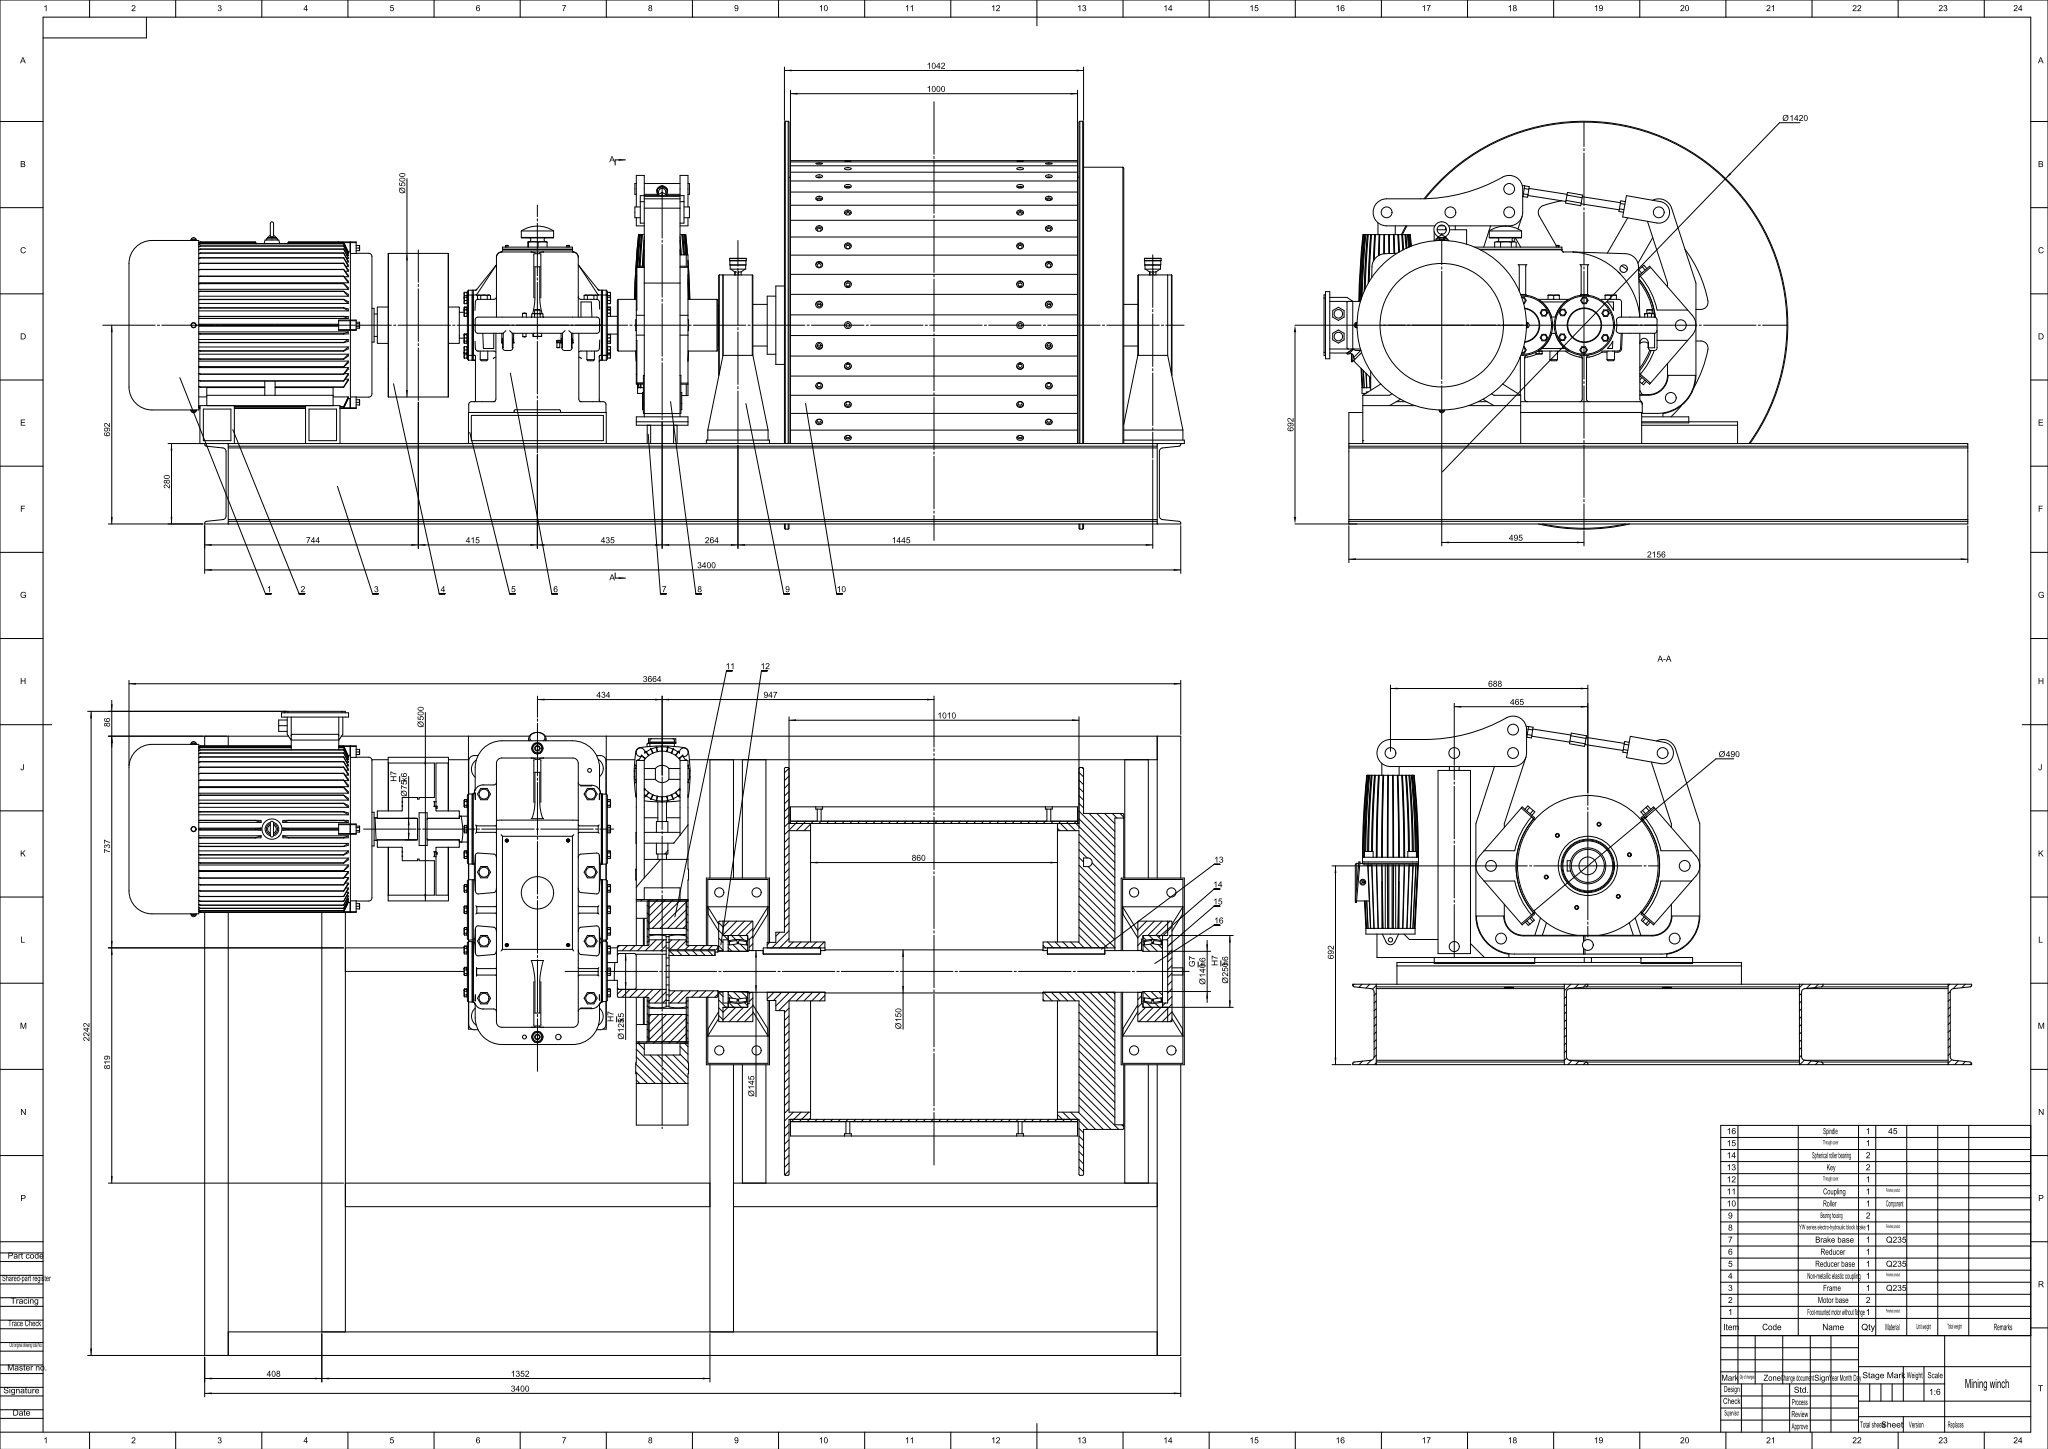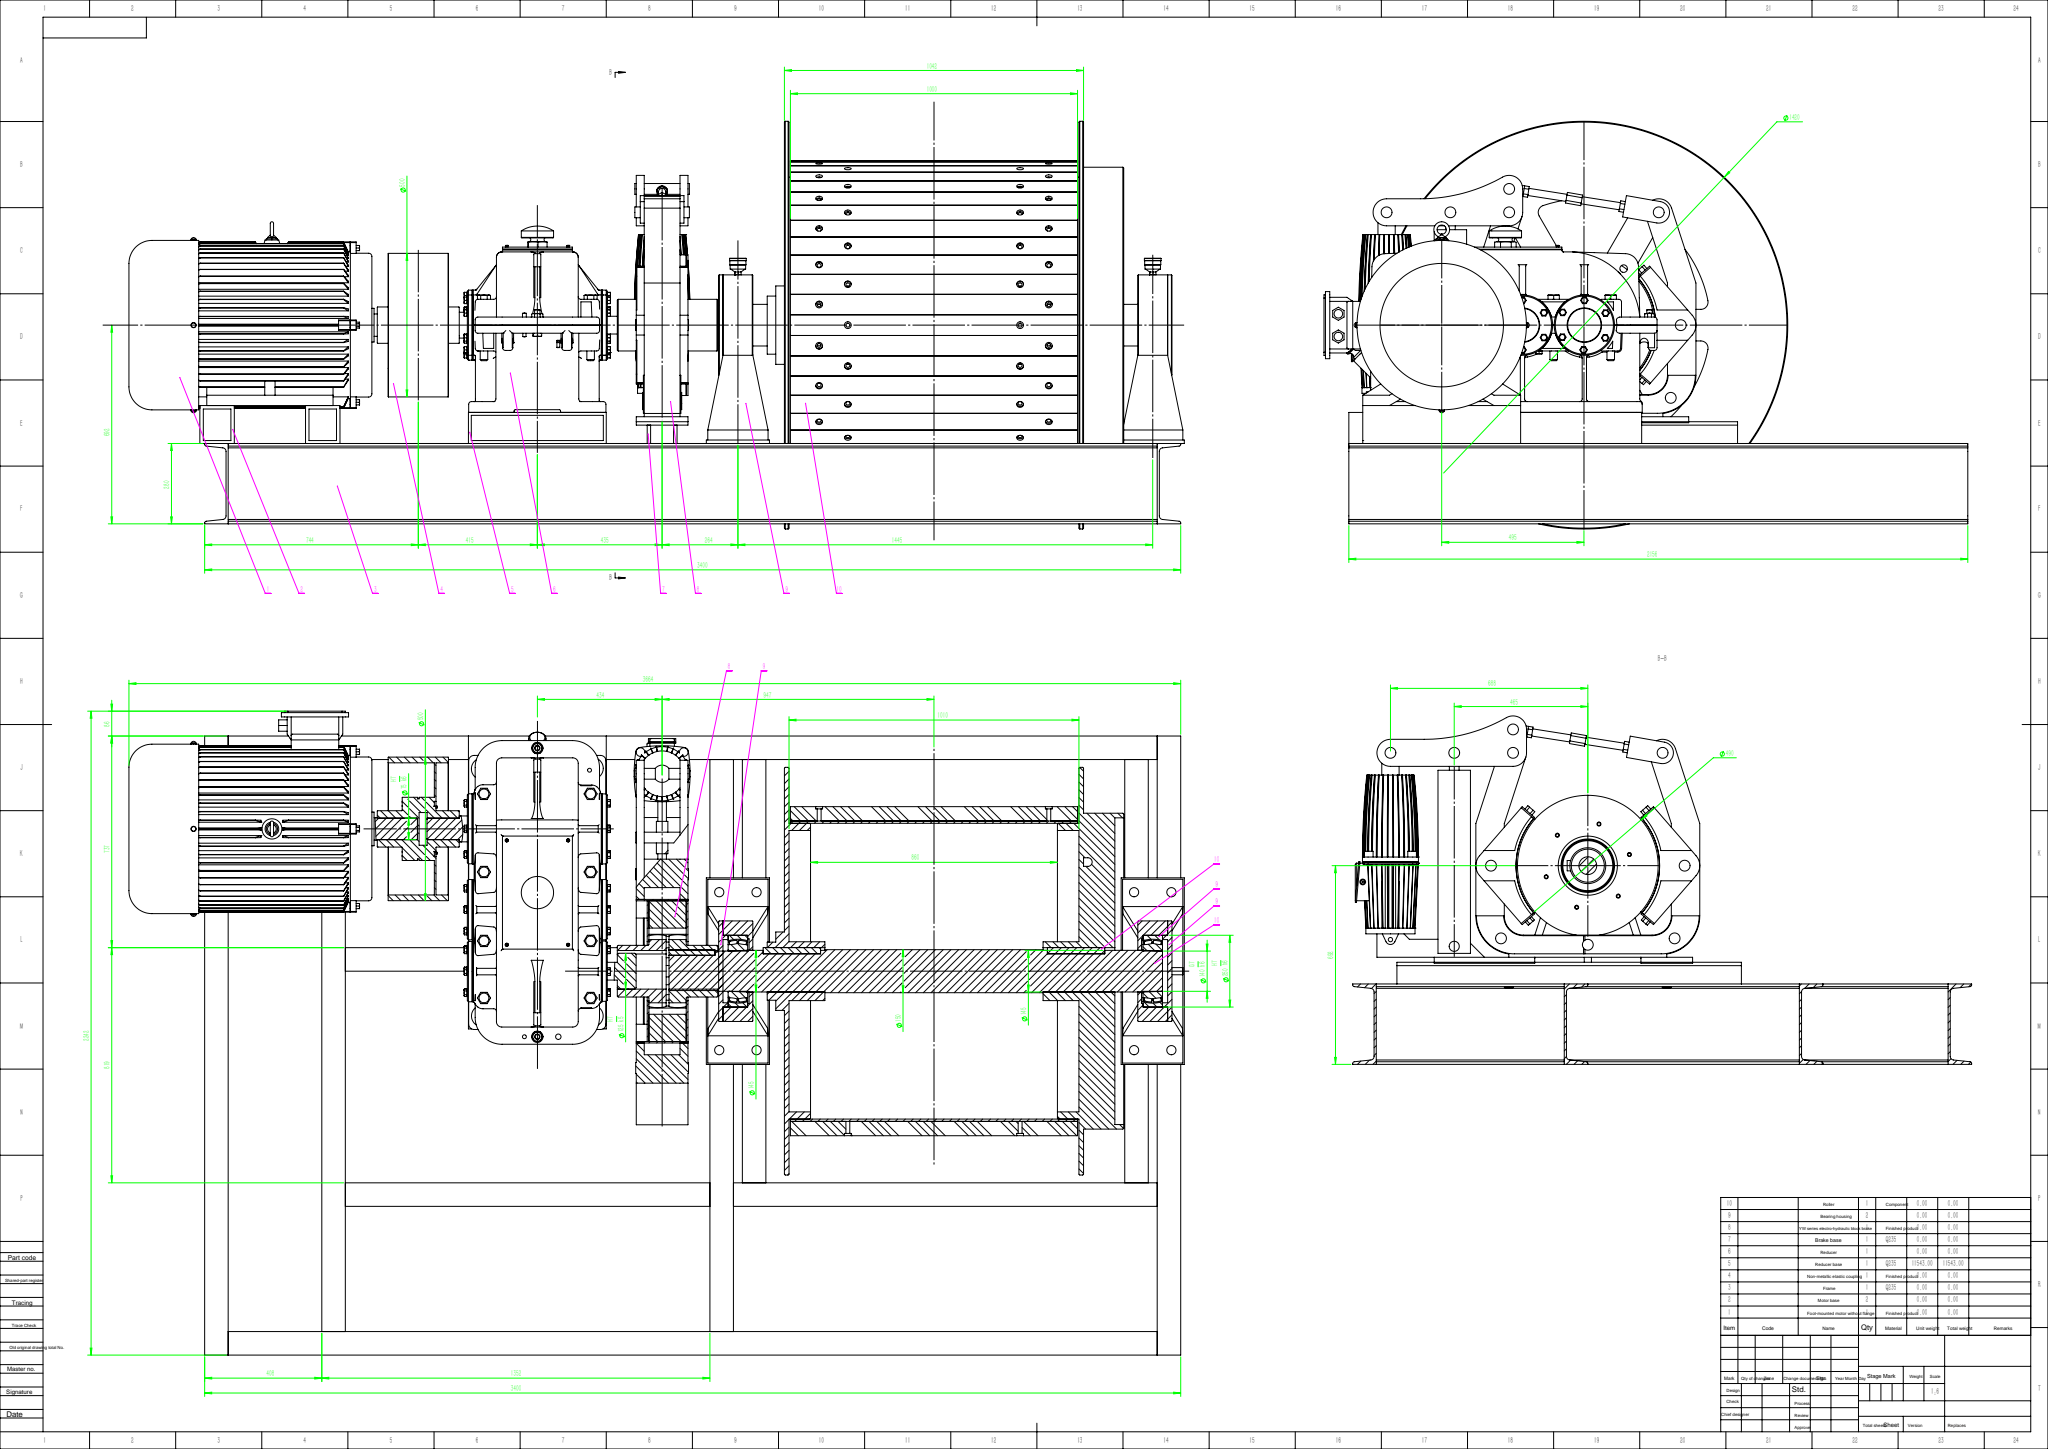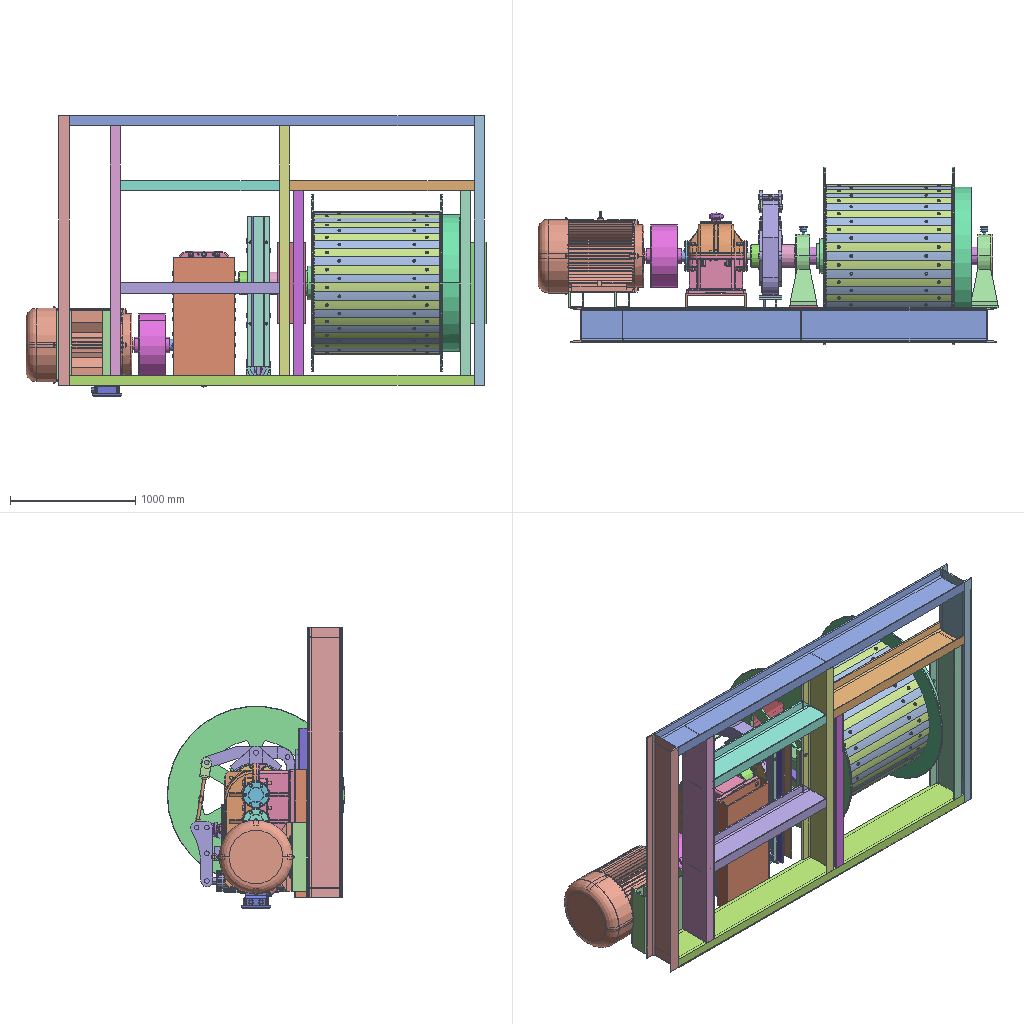Assembly | SolidWorks | 66 different items | 167 placed | box 3676 x 1420 x 2242 mm
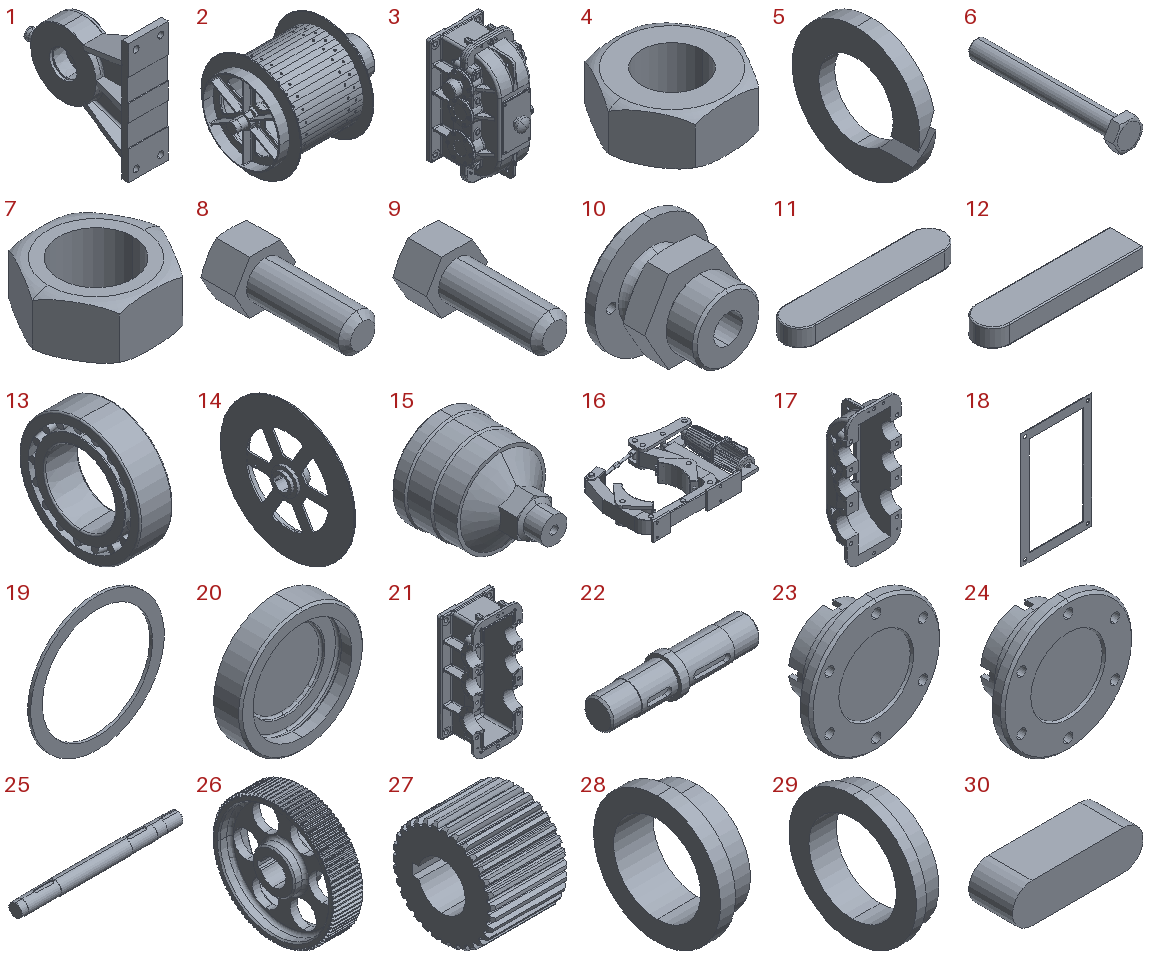Parts list (item | name | quantity | parent item | size | volume | features):
1 | (subassembly) | x2 | - | 210 x 633 x 640 mm | 18025314 mm3 | -
2 | (subassembly) | x1 | - | 1899 x 1420 x 1420 mm | 323309066 mm3 | features ReferencePattern 24, LocalCirPattern 1
3 | (subassembly) | x1 | - | - | 87002106 mm3 | features ReferencePattern 45, CompositeCurve 27, MirrorCompFeat 4, LocalCirPattern 3, AEMSimFeature 1
4 | - | x2 | in 3 | 38.971 x 33.75 x 15 mm | 10501 mm3 | features Extrusion 1, RevCut 1, Scale 1
5 | - | x8 | in 3 | 3 x 24 x 24 mm | 848.529 mm3 | features ICE 1, Revolution 1
6 | - | x8 | in 3 | 45.466 x 228.75 x 39.375 mm | 135169 mm3 | features Chamfer 1, Extrusion 1, ICE 1, RevCut 1, Scale 1
7 | - | x8 | in 3 | 24.249 x 21 x 10 mm | 2242 mm3 | features Extrusion 1, ICE 1, RevCut 1
8 | - | x2 | in 3 | 10 x 22 x 8.66 mm | 745.342 mm3 | features ICE 2, BlendCut 1, Chamfer 1, RevCut 1, Revolution 1
9 | - | x2 | in 3 | 10 x 22 x 8.66 mm | 755.833 mm3 | features ICE 2, Revolution 2, BlendCut 1, Chamfer 1, Fillet 1, RevCut 1
10 | - | x1 | in 3 | 90 x 69.375 x 90 mm | 178103 mm3 | features Chamfer 2, ICE 2, RevCut 1, Revolution 1, Scale 1
11 | - | x2 | in 2 | 200 x 40 x 22 mm | 168172 mm3 | features Extrusion 1, Fillet 1
12 | - | x1 | in 2 | 160 x 36 x 20 mm | 112209 mm3 | features Extrusion 1, Fillet 1
13 | - | x2 | in 1 | 68 x 250 x 250 mm | 1755852 mm3 | features Revolution 3, CirPattern 1, Fillet 1, MirrorPattern 1
14 | - | x1 | in 2 | 201 x 1420 x 1420 mm | 29509148 mm3 | features ICE 5, CirPattern 2, Chamfer 1, Fillet 1, RevCut 1, Revolution 1
15 | - | x2 | in 1 | 58 x 70 x 58 mm | 93422 mm3 | features Boss 1, Revolution 1
16 | - | x1 | - | 1200 x 861.523 x 195 mm | 52258785 mm3 | features Boss 43, Fillet 5, MirrorPattern 5, Cut 4, CombineBodies 3, CirPattern 2, Revolution 2, Extrusion 1, MirrorSolid 1
17 | - | x1 | in 3 | 446.25 x 262.5 x 1058 mm | 19685797 mm3 | features Fillet 30, ICE 30, MirrorPattern 4, RevCut 3, Revolution 3, Sculpt 2, Extrusion 1, Scale 1
18 | - | x1 | in 3 | 241.875 x 1.875 x 393.75 mm | 60360 mm3 | features Extrusion 1, Scale 1
19 | - | x1 | in 3 | 46 x 1 x 46 mm | 527.788 mm3 | features Revolution 1
20 | - | x1 | in 3 | 112.5 x 41.25 x 112.5 mm | 215843 mm3 | features Chamfer 1, Revolution 1, Scale 1
21 | - | x1 | in 3 | 478.125 x 303.75 x 1058 mm | 34791159 mm3 | features ICE 51, Fillet 41, MirrorPattern 15, Revolution 5, RevCut 4, Sculpt 3, BlendCut 1, Extrusion 1, Scale 1, SweepCut 1
22 | - | x1 | in 3 | 333.75 x 84.375 x 84.375 mm | 1222734 mm3 | features ICE 2, Chamfer 1, Revolution 1, Scale 1
23 | - | x1 | in 3 | 210 x 76.875 x 210 mm | 837773 mm3 | features ICE 2, Revolution 1, Scale 1
24 | - | x1 | in 3 | 210 x 76.875 x 210 mm | 837773 mm3 | features ICE 2, Revolution 1, Scale 1
25 | - | x1 | in 2 | 1719 x 150 x 150 mm | 28459508 mm3 | features ICE 2, Chamfer 1, Revolution 1
26 | - | x1 | in 3 | 84.375 x 348.75 x 348.75 mm | 2753310 mm3 | features Chamfer 5, ICE 3, RevCut 1, Revolution 1, Scale 1
27 | - | x1 | in 3 | 112.5 x 150.753 x 150.909 mm | 1373452 mm3 | features ICE 3, RevCut 1, Revolution 1, Scale 1
28 | - | x1 | in 3 | 16 x 51 x 51 mm | 11385 mm3 | features Revolution 1
29 | - | x1 | in 3 | 20.625 x 95.625 x 95.625 mm | 64156 mm3 | features Revolution 1, Scale 1
30 | - | x1 | in 3 | 56.25 x 18.75 x 16.875 mm | 16652 mm3 | features Extrusion 1, Scale 1
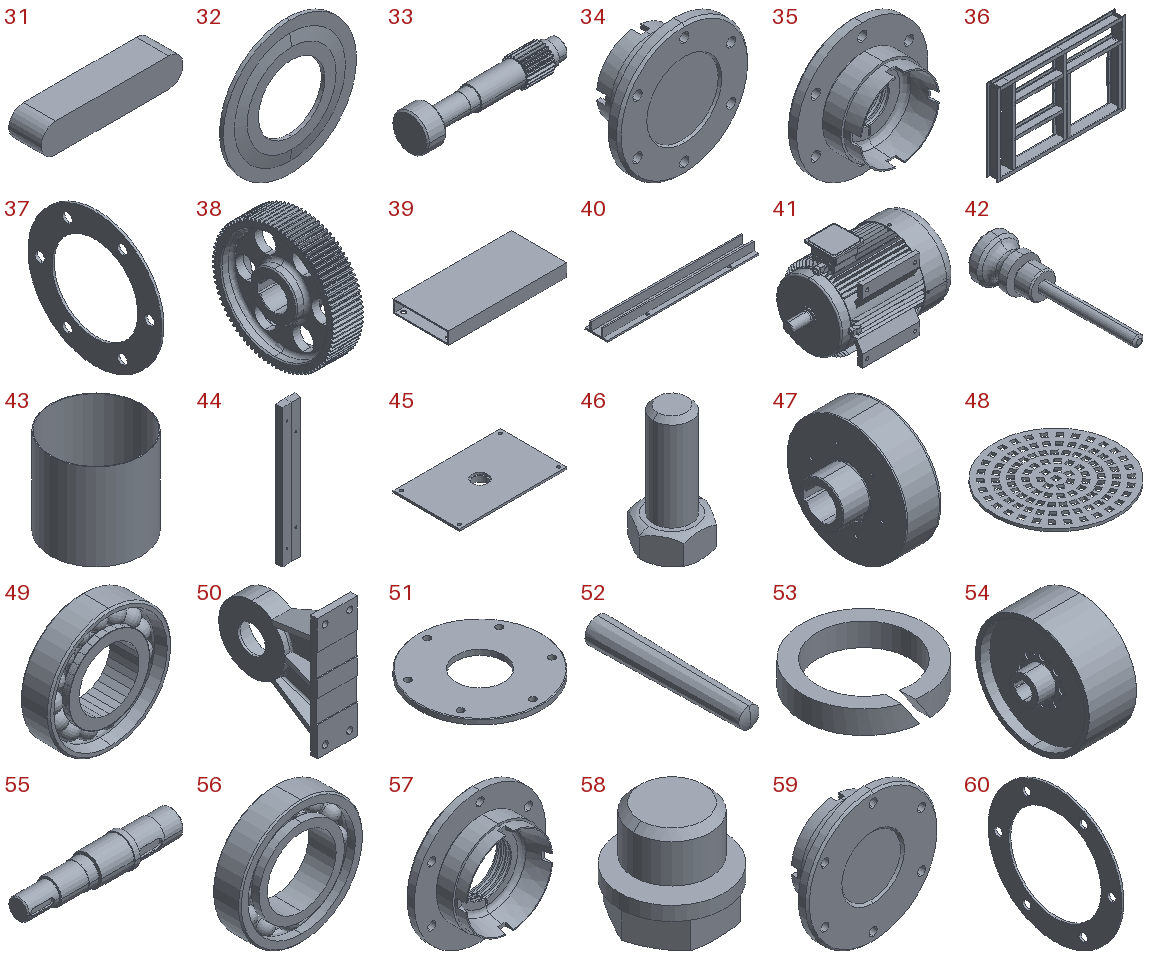31 | - | x1 | in 3 | 82.5 x 18.75 x 16.875 mm | 24958 mm3 | features Extrusion 1, Scale 1
32 | - | x2 | in 3 | 135 x 5.62 x 135 mm | 39683 mm3 | features Revolution 1, Scale 1
33 | - | x1 | in 3 | 511.875 x 125 x 125 mm | 2700404 mm3 | features ICE 4, Fillet 2, Chamfer 1, Revolution 1, Scale 1
34 | - | x1 | in 3 | 210 x 76.875 x 210 mm | 837773 mm3 | features ICE 2, Revolution 1, Scale 1
35 | - | x1 | in 3 | 210 x 76.875 x 210 mm | 727097 mm3 | features ICE 3, RevCut 1, Revolution 1, Scale 1
36 | - | x1 | - | 3413 x 292 x 2156 mm | 90885444 mm3 | features ICE 2, WeldMemberFeat 1, WeldmentFeature 1
37 | - | x4 | in 3 | 3.75 x 210 x 210 mm | 72232 mm3 | features ICE 1, Revolution 1, Scale 1
38 | - | x1 | in 3 | 103.125 x 426.489 x 426.547 mm | 6214013 mm3 | features ICE 6, Chamfer 5, Revolution 1, Scale 1
39 | - | x1 | - | 1020 x 480 x 108 mm | 11543021 mm3 | features Cut 1, Extrusion 1, Shell 1
40 | - | x1 | - | 1200 x 180 x 75.738 mm | 4409395 mm3 | features ICE 2, Extrusion 1, MirrorSolid 1, MoveFace 1
41 | - | x1 | - | 1005 x 665 x 715 mm | 186220759 mm3 | features Boss 17, Cut 5, Revolution 5, Fillet 4, Chamfer 3, CirPattern 3, RevCut 2, 3DProfileFeature 1, LPattern 1, MirrorPattern 1, MoveCopyBody 1
42 | - | x1 | in 3 | 60 x 213.75 x 60 mm | 149521 mm3 | features Revolution 1, Scale 1
43 | - | x1 | in 2 | 1046 x 1046 x 1000 mm | 26087785 mm3 | features ExtruThin 1
44 | - | x25 | in 2 | 143.632 x 54.124 x 1000 mm | 6848220 mm3 | features 3DProfileFeature 2, HoleWzd 2, MirrorPattern 2, Extrusion 1, ICE 1
45 | - | x1 | in 3 | 393.75 x 243.75 x 28.125 mm | 822488 mm3 | features ICE 3, Extrusion 1, Scale 1
46 | - | x36 | in 3 | 25.981 x 22.5 x 48.75 mm | 11356 mm3 | features Chamfer 1, Extrusion 1, ICE 1, RevCut 1, Scale 1
47 | - | x1 | in 2 | 350 x 490 x 490 mm | 25102965 mm3 | features Chamfer 3, ICE 3, HoleWzd 2, MirrorPattern 2, CirPattern 1, DelFace 1, MirrorSolid 1, MoveFace 1, RevCut 1, Revolution 1, Split 1
48 | - | x1 | in 3 | 46 x 46 x 1 mm | 1230 mm3 | features Extrusion 1
49 | - | x4 | in 3 | 135 x 32.557 x 135 mm | 1267368 mm3 | features Revolution 11, Chamfer 1, CirPattern 1, Scale 1
50 | - | x2 | in 1 | 210 x 575 x 640 mm | 14558627 mm3 | features ICE 5, HoleWzd 2, 3DProfileFeature 1, Chamfer 1, Fillet 1, MirrorPattern 1, Revolution 1
51 | - | x2 | in 1 | 350 x 350 x 33 mm | 1402702 mm3 | features ICE 2, Chamfer 1, Extrusion 1
52 | - | x2 | in 3 | 13.56 x 82.779 x 13.56 mm | 9630 mm3 | features Revolution 1, Scale 1
53 | - | x2 | in 3 | 16 x 16 x 3 mm | 255.282 mm3 | features ICE 1, Revolution 1
54 | - | x1 | - | 285.6 x 500 x 500 mm | 12150323 mm3 | features Chamfer 3, Fillet 2, Revolution 2, Boss 1, CirPattern 1, ICE 1, RevCut 1
55 | - | x1 | in 3 | 556.875 x 116.25 x 116.25 mm | 3869573 mm3 | features ICE 4, Chamfer 1, Revolution 1, Scale 1
56 | - | x2 | in 3 | 90 x 20 x 90 mm | 54381 mm3 | features Revolution 13, Chamfer 1
57 | - | x1 | in 3 | 243.75 x 71.25 x 243.75 mm | 1007577 mm3 | features ICE 3, Fillet 1, RevCut 1, Revolution 1, Scale 1
58 | - | x1 | in 3 | 56.25 x 56.25 x 52.5 mm | 84582 mm3 | features ICE 3, Chamfer 1, Extrusion 1, RevCut 1, Scale 1
59 | - | x1 | in 3 | 243.75 x 71.25 x 243.75 mm | 1137099 mm3 | features ICE 2, Chamfer 1, Revolution 1, Scale 1
60 | - | x2 | in 3 | 3.75 x 243.75 x 243.75 mm | 87142 mm3 | features ICE 1, Revolution 1, Scale 1
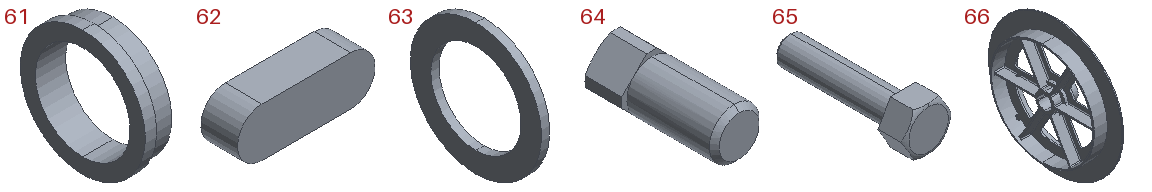61 | - | x1 | in 3 | 16 x 66 x 66 mm | 19302 mm3 | features Revolution 1
62 | - | x1 | in 3 | 45 x 12 x 16 mm | 7981 mm3 | features Extrusion 1
63 | - | x1 | in 3 | 2 x 32 x 32 mm | 848.23 mm3 | features Revolution 1
64 | - | x1 | in 3 | 12 x 25.5 x 12 mm | 2101 mm3 | features Chamfer 2, ICE 2, RevCut 1, Revolution 1
65 | - | x2 | in 3 | 33.75 x 93.75 x 29.228 mm | 33536 mm3 | features ICE 1, RevCut 1, Revolution 1, Scale 1
66 | - | x1 | in 2 | 281 x 1420 x 1420 mm | 42495584 mm3 | features ICE 5, CirPattern 2, Chamfer 1, Fillet 1, Revolution 1
Mates (type | each side: item.copy, entity, surface, feature):
In the top assembly
Coincident | 36.1 face plane Boss-Extrude1 | 50.1 face plane Boss-Extrude1
Concentric | 36.1 face cylinder Boss-Extrude1 | 50.1 face cylinder Cut-Extrude1 | 2 times
Concentric | 13.1 face cone Boss-Revolve1 | 25.1 face cylinder Revolve1
Coincident | 13.1 face plane Boss-Revolve1 | 25.1 face plane Revolve1
Coincident | 36.1 face plane Boss-Extrude1 | 50.2 face plane Boss-Extrude1
Concentric | 36.1 face cylinder Cut-Extrude1 | 50.2 face cylinder Cut-Extrude1 | 2 times
Concentric | 41.1 face cylinder Revolve1 | 54.1 face cylinder Revolve1
Coincident | 41.1 face plane Revolve1 | 54.1 face plane Revolve1
Concentric | 16.1 face cylinder Extrude25 | 47.1 face cylinder Revolve1
Coincident | 16.1 face plane Extrude20 | 47.1 face plane Mirror3
Parallel | 36.1 face plane Structural Member1 | 16.1 face plane Extrude1
Concentric | 54.1 face cylinder Revolve2 | 55.1 face cylinder Revolve1
Concentric | 16.1 edge | 40.1 edge
Coincident | 36.1 face plane Structural Member1 | 40.1 face plane Boss-Extrude2
Concentric | 16.1 face cylinder Cut-Extrude9 | 40.1 face cylinder Boss-Extrude1
Parallel | 36.1 face plane Structural Member1 | 21.1 face plane Boss-Extrude32
Coincident | 54.1 face plane Revolve1 | 55.1 face plane Revolve1
Parallel | 36.1 face plane Structural Member1 | 41.1 face plane Extrude2
Concentric | 47.1 face cylinder Revolve1 | 33.1 face cylinder Boss-Extrude2
Coincident | 47.1 face plane Revolve1 | 33.1 face plane Boss-Extrude2
Coincident | 36.1 face plane Structural Member1 | 39.1 face plane Boss-Extrude1 | 2 times
Width | 39.1 face plane Boss-Extrude1 | 39.1 face plane Boss-Extrude1 | 21.1 face plane Boss-Extrude32 | 21.1 face plane Boss-Extrude32
In subassembly 1
Concentric | 50.3 face cylinder Revolve1 | 13.2 face cylinder Base-Revolve1
Coincident | 50.3 face plane Revolve1 | 13.2 face plane Base-Revolve1
Concentric | 50.3 face cylinder M16x1.5 Tapped Hole1 | 15.1 face cylinder Revolve1
Tangent | 50.3 face cylinder Revolve1 | 15.1 face plane Extrude1
InPlace | 13.2 face plane Base-Revolve1 | 51.1 plane
In subassembly 2
Concentric | 25.2 face cylinder Revolve1 | 66.1 face cylinder Revolve1
Coincident | 25.2 face plane Revolve1 | 66.1 face plane Revolve1
Coincident | 25.2 face plane Cut-Extrude2 | 66.1 face plane Cut-Extrude4
Concentric | 25.2 face cylinder Cut-Extrude2 | 11.1 face cylinder Base-Extrude
Coincident | 25.2 face plane Cut-Extrude2 | 11.1 face plane Base-Extrude | 2 times
Coincident | 25.2 face plane Cut-Extrude2 | 11.2 face plane Base-Extrude | 2 times
Concentric | 25.2 face cylinder Cut-Extrude2 | 11.2 face cylinder Base-Extrude
Coincident | 25.2 face plane Cut-Extrude1 | 12.1 face plane Base-Extrude | 2 times
Concentric | 25.2 face cylinder Cut-Extrude1 | 12.1 face cylinder Base-Extrude
Concentric | 25.2 face cylinder Revolve1 | 47.2 face cylinder Revolve1
Coincident | 12.1 face plane Base-Extrude | 47.2 face plane Cut-Extrude1
Coincident | 25.2 face plane Revolve1 | 47.2 face plane Revolve1
Concentric | 25.2 face cylinder Revolve1 | 14.1 face cylinder Revolve1
Coincident | 11.2 face plane Base-Extrude | 14.1 face plane Cut-Extrude4
Coincident | 25.2 face plane Revolve1 | 14.1 face plane Revolve1
Concentric | 66.1 face cylinder Revolve1 | 43.1 face cylinder Extrude-Thin1
DistanceDim | 43.1 face plane Extrude-Thin1 | 66.1 face plane Revolve1
Concentric | 43.1 face cylinder Extrude-Thin1 | 44.1 face cylinder Boss-Extrude2
DistanceDim | 66.1 face plane Revolve1 | 44.1 face plane Boss-Extrude1
In subassembly 3
Coincident | 21.2 face plane Revolve2 | 37.1 face plane Revolve1
Concentric | 21.2 edge | 37.1 edge
Concentric | 21.2 face cylinder Cut-Extrude87 | 37.1 edge
Parallel | 34.1 face plane Revolve1 | 37.1 face plane Revolve1
Coincident | 34.1 edge | 37.1 edge
Concentric | 34.1 edge | 37.1 edge
Concentric | 21.2 face cylinder Cut-Extrude89 | 49.1 face cylinder Revolve1
Coincident | 34.1 face plane Revolve1 | 49.1 face plane Revolve1
Concentric | 21.2 face cylinder Cut-Extrude89 | 32.1 face cylinder Revolve1
Coincident | 49.1 face plane Revolve1 | 32.1 face plane Revolve1
Concentric | 49.1 face cylinder Revolve1 | 33.2 face cylinder Revolve1
Coincident | 32.1 face plane Revolve1 | 33.2 face plane Revolve1
Concentric | 21.2 face cylinder Cut-Extrude89 | 49.2 face cylinder Revolve1
Coincident | 33.2 face plane Revolve1 | 49.2 face plane Revolve1
Coincident | 21.2 face plane Revolve2 | 37.2 face plane Revolve1
Coincident | 21.2 face cylinder Mirror46 | 37.2 edge
Concentric | 21.2 edge | 37.2 edge
Concentric | 33.2 face cylinder Revolve1 | 35.1 face cylinder Revolve1
Coincident | 37.2 face plane Revolve1 | 35.1 face plane Revolve1
Coincident | 37.2 edge | 35.1 edge
Concentric | 21.2 face cylinder Revolve3 | 37.3 face cylinder Revolve1
Coincident | 21.2 face plane Revolve2 | 37.3 face plane Revolve1
Concentric | 21.2 face cylinder Mirror46 | 37.3 face cylinder Cut-Extrude1
Concentric | 21.2 face cylinder Revolve3 | 24.1 face cylinder Revolve1
Coincident | 37.3 face plane Revolve1 | 24.1 face plane Revolve1
Concentric | 37.3 edge | 24.1 edge
Concentric | 21.2 face cylinder Revolve3 | 49.3 face cylinder Revolve1
Coincident | 24.1 face plane Revolve1 | 49.3 face plane Revolve1
Concentric | 49.3 face cylinder Revolve1 | 32.2 face cylinder Revolve1
Coincident | 49.3 face plane Revolve1 | 32.2 face plane Revolve1
Concentric | 49.3 face cylinder Revolve1 | 22.1 face cylinder Revolve1
Coincident | 49.3 face plane Revolve1 | 22.1 face plane Revolve1
Coincident | 32.2 face plane Revolve1 | 29.1 face plane Revolve1
Concentric | 22.1 face cylinder Revolve1 | 29.1 face cylinder Revolve1
Coincident | 22.1 face plane Boss-Extrude1 | 31.1 face plane Boss-Extrude1
Concentric | 22.1 face cylinder Cut-Extrude1 | 31.1 face cylinder Boss-Extrude1
Coincident | 22.1 face plane Boss-Extrude1 | 30.1 face plane Boss-Extrude1
Coincident | 22.1 face plane Cut-Extrude1 | 30.1 face plane Boss-Extrude1
Concentric | 22.1 face cylinder Cut-Extrude1 | 30.1 face cylinder Boss-Extrude1
Coincident | 31.1 face plane Boss-Extrude1 | 27.1 face plane Cut-Extrude7
Coincident | 29.1 face plane Revolve1 | 27.1 face plane Revolve1
Coincident | 30.1 face plane Boss-Extrude1 | 26.1 face plane Cut-Extrude6 | 2 times
Tangent | 33.2 face cylinder Cut-Extrude2 | 26.1 face cylinder Cut-Extrude5
Concentric | 22.1 face cylinder Revolve1 | 28.1 face cylinder Revolve1
Coincident | 26.1 face plane Revolve1 | 28.1 face plane Revolve1
Concentric | 22.1 face cylinder Revolve1 | 49.4 face cylinder Revolve1
Coincident | 28.1 face plane Revolve1 | 49.4 face plane Revolve1
Coincident | 21.2 face plane Revolve2 | 37.4 face plane Revolve1
Coincident | 21.2 edge | 37.4 edge
Concentric | 21.2 face cylinder Cut-Extrude87 | 37.4 face cylinder Cut-Extrude1
Concentric | 21.2 face cylinder Revolve3 | 23.1 face cylinder Revolve1
Coincident | 37.4 face plane Revolve1 | 23.1 face plane Revolve1
Concentric | 37.4 edge | 23.1 edge
Coincident | 21.2 face plane Revolve4 | 60.1 face plane Revolve1
Concentric | 21.2 edge | 60.1 edge
Concentric | 21.2 face cylinder Revolve4 | 59.1 face cylinder Revolve1
Coincident | 59.1 face plane Revolve1 | 60.1 face plane Revolve1
Concentric | 59.1 face cylinder Cut-Extrude2 | 60.1 face cylinder Cut-Extrude1
Concentric | 21.2 face cylinder Revolve4 | 56.1 face cylinder Revolve1
Coincident | 59.1 face plane Revolve1 | 56.1 face plane Revolve1
Coincident | 56.1 face plane Revolve1 | 61.1 face plane Revolve1
Concentric | 56.1 face cylinder Revolve1 | 61.1 face cylinder Revolve1
Concentric | 61.1 face cylinder Revolve1 | 55.2 face cylinder Revolve1
Coincident | 56.1 face plane Revolve1 | 55.2 face plane Revolve1
Coincident | 55.2 face plane Boss-Extrude2 | 62.1 face plane Boss-Extrude1
Concentric | 55.2 face cylinder Cut-Extrude3 | 62.1 face cylinder Boss-Extrude1
Parallel | 62.1 face plane Boss-Extrude1 | 38.1 face plane Cut-Extrude8
Coincident | 61.1 face plane Revolve1 | 38.1 face plane Revolve1
Coincident | 56.2 face plane Revolve1 | 55.2 face plane Revolve1
Concentric | 56.2 face cylinder Revolve1 | 55.2 face cylinder Revolve1
Coincident | 21.2 face plane Revolve4 | 60.2 face plane Revolve1
Coincident | 21.2 face cylinder Cut-Extrude87 | 60.2 edge
Coincident | 60.2 face plane Revolve1 | 57.1 face plane Revolve1
Coincident | 60.2 face cylinder Cut-Extrude1 | 57.1 edge
Concentric | 21.2 face cylinder Cut-Extrude87 | 57.1 face cylinder Cut-Extrude3
Coincident | 37.2 face plane Revolve1 | 17.1 face plane Revolve2
Coincident | 17.1 face plane Boss-Extrude2 | 18.1 face plane Boss-Extrude1
Concentric | 17.1 face cylinder Cut-Extrude39 | 18.1 face cylinder Boss-Extrude1
Coincident | 18.1 face plane Boss-Extrude1 | 45.1 face plane Boss-Extrude1 | 2 times
Concentric | 18.1 face cylinder Boss-Extrude1 | 45.1 face cylinder Boss-Extrude1
Concentric | 45.1 face cylinder Cut-Extrude1 | 10.1 face cylinder Revolve2
Coincident | 45.1 face plane Boss-Extrude1 | 10.1 face plane Revolve2
Coincident | 10.1 face plane Revolve2 | 48.1 face plane Boss-Extrude1
Concentric | 10.1 face cylinder Revolve2 | 48.1 face cylinder Boss-Extrude1
Coincident | 48.1 face plane Boss-Extrude1 | 19.1 face plane Revolve1
Concentric | 48.1 face cylinder Boss-Extrude1 | 19.1 face cylinder Revolve1
Coincident | 10.1 face plane Revolve2 | 20.1 face plane Revolve1
Concentric | 10.1 face cylinder Revolve2 | 20.1 face cylinder Revolve1
Coincident | 21.2 face plane Revolve6 | 42.1 face plane Revolve1
Concentric | 21.2 face cylinder Revolve6 | 42.1 face cylinder Revolve1
Coincident | 17.1 face plane Intersect 3 | 6.1 face plane Boss-Extrude1
Concentric | 17.1 face cylinder Cut-Extrude44 | 6.1 face cylinder Boss-Extrude2
Concentric | 17.1 face cylinder Cut-Revolve2 | 64.1 face cylinder Revolve1
Coincident | 35.1 face plane Revolve1 | 46.1 face plane Boss-Extrude1
Concentric | 21.2 face cylinder Revolve5 | 63.1 face cylinder Revolve1
Concentric | 21.2 face cylinder Revolve5 | 58.1 face cylinder Boss-Extrude5
Coincident | 63.1 face plane Revolve1 | 58.1 face plane Boss-Extrude2
Coincident | 59.1 face plane Revolve1 | 46.2 face plane Boss-Extrude1
Concentric | 59.1 face cylinder Cut-Extrude2 | 46.2 face cylinder Boss-Extrude2
Coincident | 21.2 face plane Intersect 4 | 7.1 face plane Boss-Extrude1
Coincident | 6.1 face cylinder Boss-Extrude2 | 7.1 edge
Coincident | 17.1 face plane Intersect 3 | 6.2 face plane Boss-Extrude1
Coincident | 21.2 face plane Intersect 4 | 7.2 face plane Boss-Extrude1
Concentric | 6.3 face cylinder Boss-Extrude2 | 7.2 face cylinder Cut-Extrude1
Coincident | 21.2 face plane Intersect 4 | 7.3 face plane Boss-Extrude1
Concentric | 6.4 face cylinder Boss-Extrude2 | 7.3 face cylinder Cut-Extrude1
Coincident | 5.1 face plane Revolve1 | 7.4 face plane Boss-Extrude1
Concentric | 6.2 face cylinder Boss-Extrude2 | 7.4 face cylinder Cut-Extrude1
Coincident | 17.1 face plane Cut-Extrude43 | 53.1 face plane Revolve1
Concentric | 17.1 face cylinder Cut-Extrude42 | 53.1 face cylinder Revolve1
Coincident | 53.1 face plane Revolve1 | 4.1 face plane Boss-Extrude2
Concentric | 53.1 face cylinder Revolve1 | 4.1 face cylinder Boss-Extrude2
Coincident | 21.2 face plane Cut-Extrude43 | 65.1 face plane Revolve1
Concentric | 21.2 face cylinder Cut-Extrude42 | 65.1 face cylinder Revolve1
Coincident | 45.1 face plane Boss-Extrude1 | 9.1 face plane Revolve1
Concentric | 45.1 face cylinder Boss-Extrude1 | 9.1 face cylinder Revolve1
Coincident | 45.1 face plane Boss-Extrude1 | 8.1 face plane Revolve1
Concentric | 45.1 face cylinder Boss-Extrude1 | 8.1 face cylinder Revolve1
Coincident | 45.1 face plane Boss-Extrude1 | 8.2 face plane Revolve1
Concentric | 45.1 face cylinder Boss-Extrude1 | 8.2 face cylinder Revolve1
Coincident | 45.1 face plane Boss-Extrude1 | 9.2 face plane Revolve1
Concentric | 45.1 face cylinder Boss-Extrude1 | 9.2 face cylinder Revolve1
Coincident | 17.1 face plane Cut-Extrude50 | 53.2 face plane Revolve1
Concentric | 17.1 face cylinder Cut-Extrude50 | 53.2 face cylinder Revolve1
Coincident | 53.2 face plane Revolve1 | 4.2 face plane Boss-Extrude2
Concentric | 53.2 face cylinder Revolve1 | 4.2 face cylinder Boss-Extrude2
Coincident | 21.2 face plane Cut-Extrude91 | 65.2 face plane Revolve1
Concentric | 21.2 face cylinder Cut-Extrude44 | 65.2 face cylinder Revolve1
Concentric | 17.1 face cone Cut-Revolve3 | 52.1 face cone Revolve1
Coincident | 17.1 edge | 52.1 face cone Revolve1
Concentric | 49.3 face cylinder Revolve1 | 27.1 face cylinder Boss-Extrude1